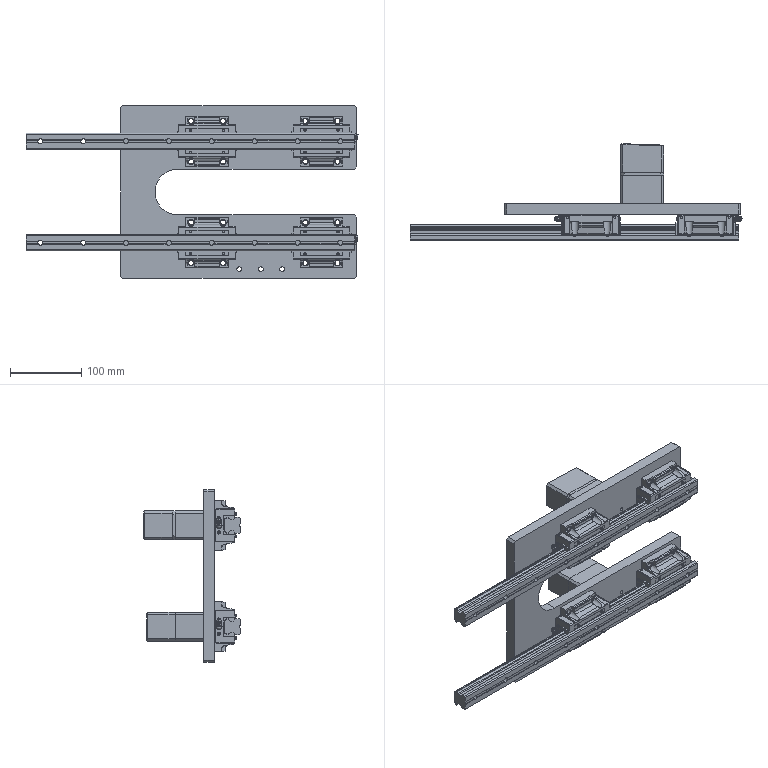Part | SolidWorks | 16 solids | 1830 faces | box 464.6 x 134.966 x 242 mm | volume 2038560 mm3 | plane 1001 | cylinder 543 | cone 174 | torus 88 | sphere 24 | commonest cylinder face diameters 11 x72 10 x48 8 x40 6.8 x38 3 x32 3.518 x32